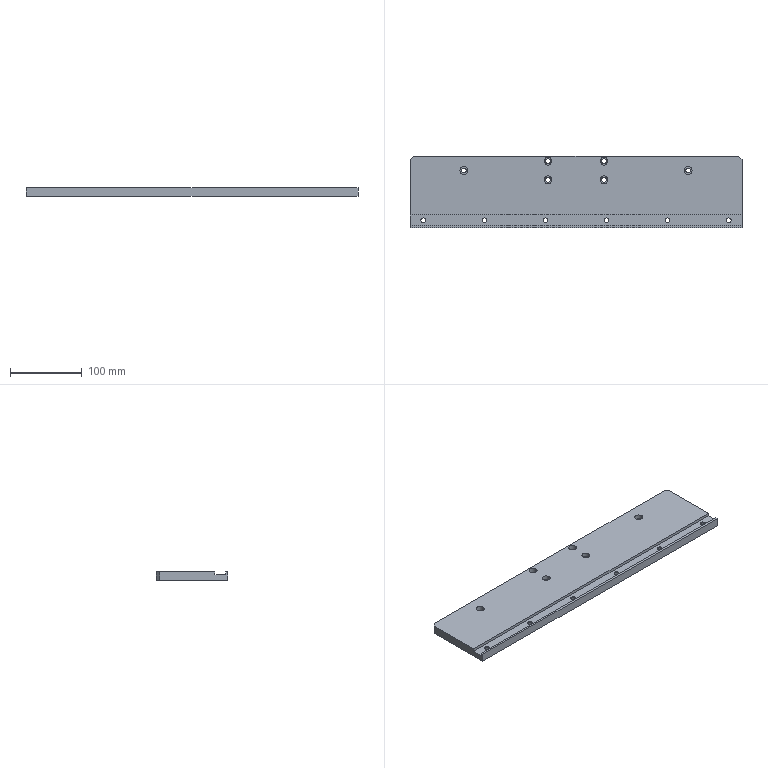Part | SolidWorks | features HoleWzd 3, Chamfer 1, Cut 1, Extrusion 1, ICE 1 | 1 solid | 78 faces | box 462 x 100 x 12 mm | volume 516299 mm3 | cylinder 52 | plane 26 | commonest cylinder face diameters 6.6 x24 11 x24 20 x4